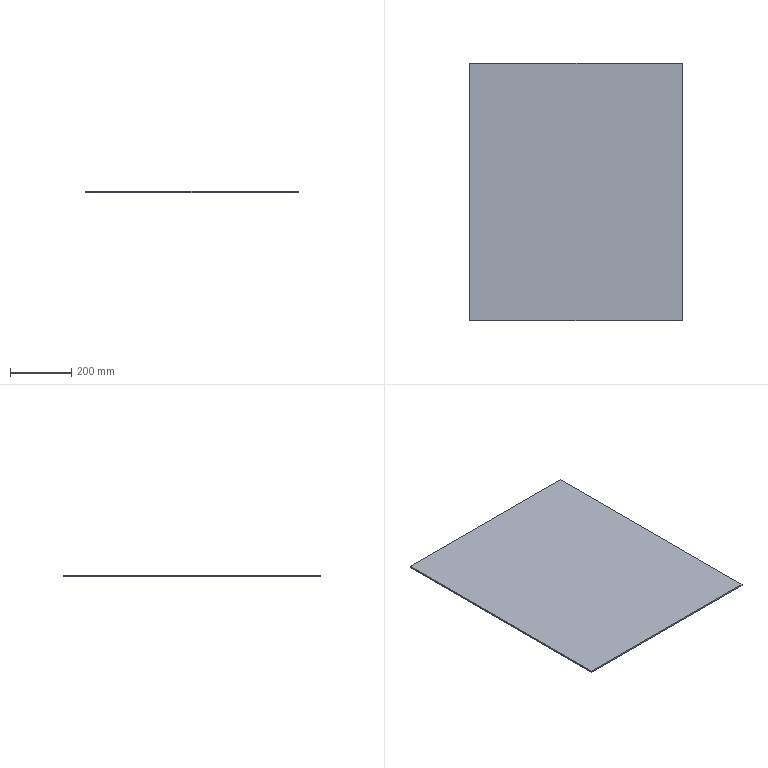Part | SolidWorks | features Extrusion 1, HoleWzd 1 | 1 solid | 6 faces | box 696 x 842 x 5 mm | volume 2930160 mm3 | plane 6
STEP:
#1=CARTESIAN_POINT('',(348.,-421.,0.));
#2=VERTEX_POINT('',#1);
#3=CARTESIAN_POINT('',(348.,421.,0.));
#4=VERTEX_POINT('',#3);
#5=CARTESIAN_POINT('',(348.,421.,0.));
#6=DIRECTION('',(0.,1.,0.));
#7=VECTOR('',#6,1000.);
#8=LINE('',#5,#7);
#9=EDGE_CURVE('',#2,#4,#8,.T.);
#10=ORIENTED_EDGE('',*,*,#9,.T.);
#11=CARTESIAN_POINT('',(348.,421.,5.));
#12=VERTEX_POINT('',#11);
#13=CARTESIAN_POINT('',(348.,421.,5.));
#14=DIRECTION('',(0.,0.,-1.));
#15=VECTOR('',#14,1000.);
#16=LINE('',#13,#15);
#17=EDGE_CURVE('',#12,#4,#16,.T.);
#18=ORIENTED_EDGE('',*,*,#17,.F.);
#19=CARTESIAN_POINT('',(348.,-421.,5.));
#20=VERTEX_POINT('',#19);
#21=CARTESIAN_POINT('',(348.,421.,5.));
#22=DIRECTION('',(0.,1.,0.));
#23=VECTOR('',#22,1000.);
#24=LINE('',#21,#23);
#25=EDGE_CURVE('',#20,#12,#24,.T.);
#26=ORIENTED_EDGE('',*,*,#25,.F.);
#27=CARTESIAN_POINT('',(348.,-421.,5.));
#28=DIRECTION('',(0.,0.,-1.));
#29=VECTOR('',#28,1000.);
#30=LINE('',#27,#29);
#31=EDGE_CURVE('',#20,#2,#30,.T.);
#32=ORIENTED_EDGE('',*,*,#31,.T.);
#33=EDGE_LOOP('',(#10,#18,#26,#32));
#34=FACE_OUTER_BOUND('',#33,.T.);
#35=CARTESIAN_POINT('',(348.,421.,5.));
#36=DIRECTION('',(-1.,0.,0.));
#37=DIRECTION('',(0.,-1.,0.));
#38=AXIS2_PLACEMENT_3D('',#35,#36,#37);
#39=PLANE('',#38);
#40=ADVANCED_FACE('',(#34),#39,.F.);
#41=CARTESIAN_POINT('',(-348.,421.,0.));
#42=VERTEX_POINT('',#41);
#43=CARTESIAN_POINT('',(-348.,421.,0.));
#44=DIRECTION('',(-1.,0.,0.));
#45=VECTOR('',#44,1000.);
#46=LINE('',#43,#45);
#47=EDGE_CURVE('',#4,#42,#46,.T.);
#48=ORIENTED_EDGE('',*,*,#47,.T.);
#49=CARTESIAN_POINT('',(-348.,421.,5.));
#50=VERTEX_POINT('',#49);
#51=CARTESIAN_POINT('',(-348.,421.,5.));
#52=DIRECTION('',(0.,0.,-1.));
#53=VECTOR('',#52,1000.);
#54=LINE('',#51,#53);
#55=EDGE_CURVE('',#50,#42,#54,.T.);
#56=ORIENTED_EDGE('',*,*,#55,.F.);
#57=CARTESIAN_POINT('',(-348.,421.,5.));
#58=DIRECTION('',(-1.,0.,0.));
#59=VECTOR('',#58,1000.);
#60=LINE('',#57,#59);
#61=EDGE_CURVE('',#12,#50,#60,.T.);
#62=ORIENTED_EDGE('',*,*,#61,.F.);
#63=ORIENTED_EDGE('',*,*,#17,.T.);
#64=EDGE_LOOP('',(#48,#56,#62,#63));
#65=FACE_OUTER_BOUND('',#64,.T.);
#66=CARTESIAN_POINT('',(-348.,421.,5.));
#67=DIRECTION('',(0.,-1.,0.));
#68=DIRECTION('',(0.,0.,-1.));
#69=AXIS2_PLACEMENT_3D('',#66,#67,#68);
#70=PLANE('',#69);
#71=ADVANCED_FACE('',(#65),#70,.F.);
#72=CARTESIAN_POINT('',(-348.,-421.,0.));
#73=VERTEX_POINT('',#72);
#74=CARTESIAN_POINT('',(-348.,421.,0.));
#75=DIRECTION('',(0.,-1.,0.));
#76=VECTOR('',#75,1000.);
#77=LINE('',#74,#76);
#78=EDGE_CURVE('',#42,#73,#77,.T.);
#79=ORIENTED_EDGE('',*,*,#78,.T.);
#80=CARTESIAN_POINT('',(-348.,-421.,5.));
#81=VERTEX_POINT('',#80);
#82=CARTESIAN_POINT('',(-348.,-421.,5.));
#83=DIRECTION('',(0.,0.,-1.));
#84=VECTOR('',#83,1000.);
#85=LINE('',#82,#84);
#86=EDGE_CURVE('',#81,#73,#85,.T.);
#87=ORIENTED_EDGE('',*,*,#86,.F.);
#88=CARTESIAN_POINT('',(-348.,421.,5.));
#89=DIRECTION('',(0.,-1.,0.));
#90=VECTOR('',#89,1000.);
#91=LINE('',#88,#90);
#92=EDGE_CURVE('',#50,#81,#91,.T.);
#93=ORIENTED_EDGE('',*,*,#92,.F.);
#94=ORIENTED_EDGE('',*,*,#55,.T.);
#95=EDGE_LOOP('',(#79,#87,#93,#94));
#96=FACE_OUTER_BOUND('',#95,.T.);
#97=CARTESIAN_POINT('',(-348.,421.,5.));
#98=DIRECTION('',(1.,0.,0.));
#99=DIRECTION('',(0.,1.,0.));
#100=AXIS2_PLACEMENT_3D('',#97,#98,#99);
#101=PLANE('',#100);
#102=ADVANCED_FACE('',(#96),#101,.F.);
#103=CARTESIAN_POINT('',(-348.,-421.,0.));
#104=DIRECTION('',(1.,0.,0.));
#105=VECTOR('',#104,1000.);
#106=LINE('',#103,#105);
#107=EDGE_CURVE('',#73,#2,#106,.T.);
#108=ORIENTED_EDGE('',*,*,#107,.T.);
#109=ORIENTED_EDGE('',*,*,#31,.F.);
#110=CARTESIAN_POINT('',(-348.,-421.,5.));
#111=DIRECTION('',(1.,0.,0.));
#112=VECTOR('',#111,1000.);
#113=LINE('',#110,#112);
#114=EDGE_CURVE('',#81,#20,#113,.T.);
#115=ORIENTED_EDGE('',*,*,#114,.F.);
#116=ORIENTED_EDGE('',*,*,#86,.T.);
#117=EDGE_LOOP('',(#108,#109,#115,#116));
#118=FACE_OUTER_BOUND('',#117,.T.);
#119=CARTESIAN_POINT('',(-348.,-421.,5.));
#120=DIRECTION('',(0.,1.,0.));
#121=DIRECTION('',(0.,0.,1.));
#122=AXIS2_PLACEMENT_3D('',#119,#120,#121);
#123=PLANE('',#122);
#124=ADVANCED_FACE('',(#118),#123,.F.);
#125=ORIENTED_EDGE('',*,*,#25,.T.);
#126=ORIENTED_EDGE('',*,*,#61,.T.);
#127=ORIENTED_EDGE('',*,*,#92,.T.);
#128=ORIENTED_EDGE('',*,*,#114,.T.);
#129=EDGE_LOOP('',(#125,#126,#127,#128));
#130=FACE_OUTER_BOUND('',#129,.T.);
#131=CARTESIAN_POINT('',(0.,0.,5.));
#132=DIRECTION('',(0.,0.,1.));
#133=DIRECTION('',(1.,0.,0.));
#134=AXIS2_PLACEMENT_3D('',#131,#132,#133);
#135=PLANE('',#134);
#136=ADVANCED_FACE('',(#130),#135,.T.);
#137=ORIENTED_EDGE('',*,*,#9,.F.);
#138=ORIENTED_EDGE('',*,*,#107,.F.);
#139=ORIENTED_EDGE('',*,*,#78,.F.);
#140=ORIENTED_EDGE('',*,*,#47,.F.);
#141=EDGE_LOOP('',(#137,#138,#139,#140));
#142=FACE_OUTER_BOUND('',#141,.T.);
#143=CARTESIAN_POINT('',(0.,0.,0.));
#144=DIRECTION('',(0.,0.,1.));
#145=DIRECTION('',(1.,0.,0.));
#146=AXIS2_PLACEMENT_3D('',#143,#144,#145);
#147=PLANE('',#146);
#148=ADVANCED_FACE('',(#142),#147,.F.);
#149=CLOSED_SHELL('',(#40,#71,#102,#124,#136,#148));
#150=MANIFOLD_SOLID_BREP('',#149);
#151=CARTESIAN_POINT('',(0.,0.,0.));
#152=DIRECTION('',(0.,0.,1.));
#153=DIRECTION('',(1.,0.,0.));
#154=AXIS2_PLACEMENT_3D('',#151,#152,#153);
#155=(LENGTH_UNIT()NAMED_UNIT(*)SI_UNIT(.MILLI.,.METRE.));
#156=UNCERTAINTY_MEASURE_WITH_UNIT(LENGTH_MEASURE(0.00001),#155,'','');
#157=(NAMED_UNIT(*)PLANE_ANGLE_UNIT()SI_UNIT($,.RADIAN.));
#158=(NAMED_UNIT(*)SI_UNIT($,.STERADIAN.)SOLID_ANGLE_UNIT());
#159=(GEOMETRIC_REPRESENTATION_CONTEXT(3)GLOBAL_UNCERTAINTY_ASSIGNED_CONTEXT((#156))GLOBAL_UNIT_ASSIGNED_CONTEXT((#155,#157,#158))REPRESENTATION_CONTEXT('',''));
#160=ADVANCED_BREP_SHAPE_REPRESENTATION('',(#150,#154),#159);